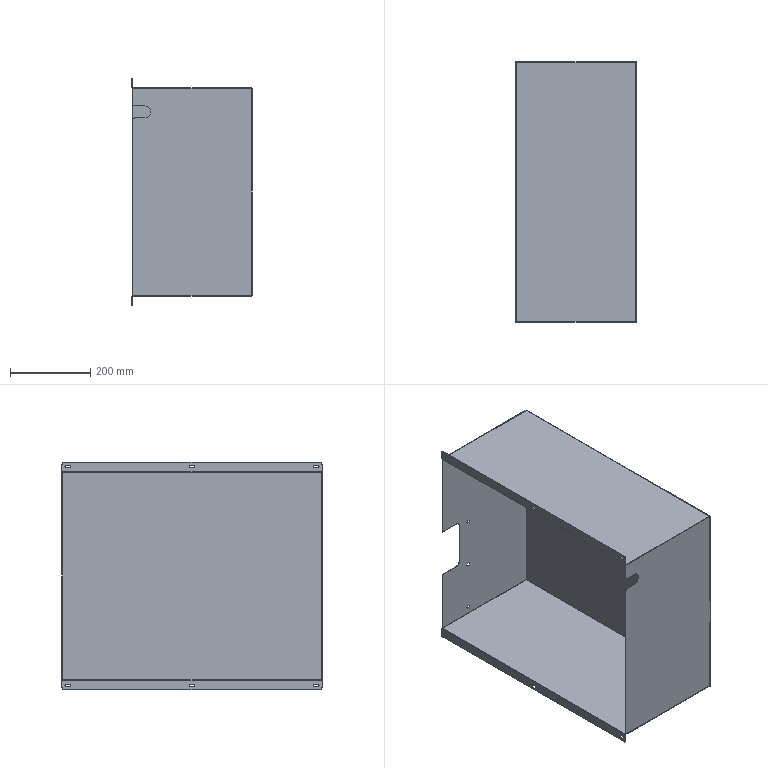Part | SolidWorks | features BaseBody 3 | 3 solids | 112 faces | box 300 x 650 x 567.6 mm | volume 1264663 mm3 | plane 79 | cylinder 33 | commonest cylinder face diameters 7 x12 1 x8 10 x6 3.4 x4 20 x2 30 x1